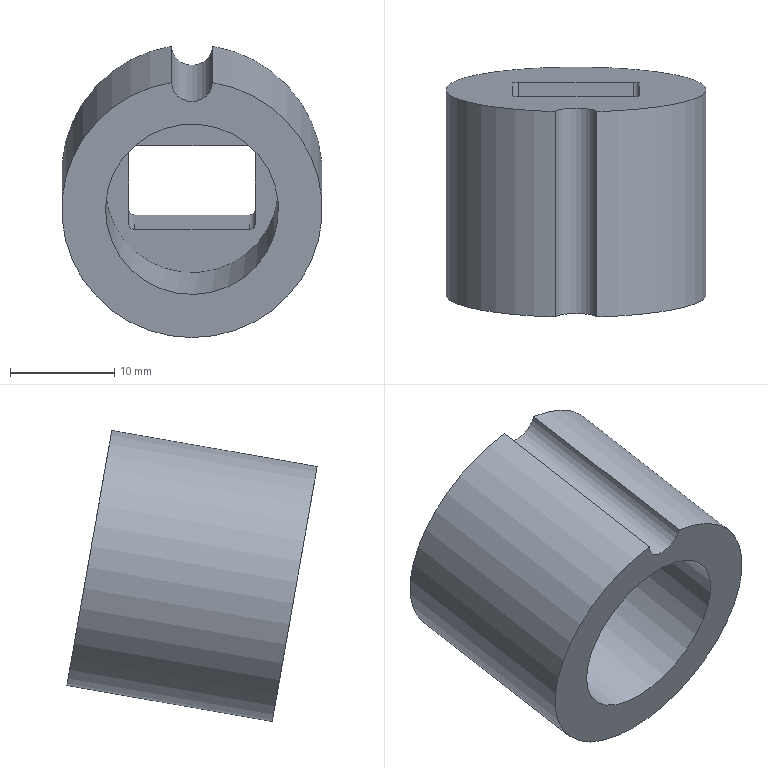Part | NX | features solid 2 | 1 solid | 14 faces | box 25 x 24.01 x 27.936 mm | volume 6304 mm3 | plane 7 | cylinder 7 | commonest cylinder face diameters 1.18 x4 4 x1 16.6 x1 25 x1
STEP:
#1=CARTESIAN_POINT('',(85.217,-526.176,-22.03));
#2=VERTEX_POINT('',#1);
#3=CARTESIAN_POINT('',(81.23,-526.176,-22.03));
#4=VERTEX_POINT('',#3);
#5=CARTESIAN_POINT('',(83.224,-526.203,-21.873));
#6=DIRECTION('',(0.,0.9848,0.1736));
#7=DIRECTION('',(-0.9972,0.01308,-0.07416));
#8=AXIS2_PLACEMENT_3D('',#5,#6,#7);
#9=CIRCLE('',#8,2.);
#10=EDGE_CURVE('',#2,#4,#9,.T.);
#11=ORIENTED_EDGE('',*,*,#10,.F.);
#12=CARTESIAN_POINT('',(83.224,-524.033,-34.183));
#13=DIRECTION('',(0.,0.9848,0.1736));
#14=DIRECTION('',(-0.9972,0.01308,-0.07416));
#15=AXIS2_PLACEMENT_3D('',#12,#13,#14);
#16=CIRCLE('',#15,12.5);
#17=EDGE_CURVE('',#2,#4,#16,.T.);
#18=ORIENTED_EDGE('',*,*,#17,.T.);
#19=EDGE_LOOP('',(#11,#18));
#20=FACE_BOUND('',#19,.T.);
#21=CARTESIAN_POINT('',(77.724,-524.743,-30.155));
#22=VERTEX_POINT('',#21);
#23=CARTESIAN_POINT('',(77.134,-524.641,-30.736));
#24=VERTEX_POINT('',#23);
#25=CARTESIAN_POINT('',(77.724,-524.641,-30.736));
#26=DIRECTION('',(0.,-0.9848,-0.1736));
#27=DIRECTION('',(0.,-0.1736,0.9848));
#28=AXIS2_PLACEMENT_3D('',#25,#26,#27);
#29=CIRCLE('',#28,0.59);
#30=EDGE_CURVE('',#22,#24,#29,.T.);
#31=ORIENTED_EDGE('',*,*,#30,.T.);
#32=CARTESIAN_POINT('',(77.134,-523.425,-37.63));
#33=VERTEX_POINT('',#32);
#34=CARTESIAN_POINT('',(77.134,-524.033,-34.183));
#35=DIRECTION('',(0.,-0.1736,0.9848));
#36=VECTOR('',#35,1000.);
#37=LINE('',#34,#36);
#38=EDGE_CURVE('',#33,#24,#37,.T.);
#39=ORIENTED_EDGE('',*,*,#38,.F.);
#40=CARTESIAN_POINT('',(77.724,-523.323,-38.211));
#41=VERTEX_POINT('',#40);
#42=CARTESIAN_POINT('',(77.724,-523.425,-37.63));
#43=DIRECTION('',(0.,-0.9848,-0.1736));
#44=DIRECTION('',(0.,-0.1736,0.9848));
#45=AXIS2_PLACEMENT_3D('',#42,#43,#44);
#46=CIRCLE('',#45,0.59);
#47=EDGE_CURVE('',#33,#41,#46,.T.);
#48=ORIENTED_EDGE('',*,*,#47,.T.);
#49=CARTESIAN_POINT('',(88.724,-523.323,-38.211));
#50=VERTEX_POINT('',#49);
#51=CARTESIAN_POINT('',(83.224,-523.323,-38.211));
#52=DIRECTION('',(-1.,0.,0.));
#53=VECTOR('',#52,1000.);
#54=LINE('',#51,#53);
#55=EDGE_CURVE('',#50,#41,#54,.T.);
#56=ORIENTED_EDGE('',*,*,#55,.F.);
#57=CARTESIAN_POINT('',(89.314,-523.425,-37.63));
#58=VERTEX_POINT('',#57);
#59=CARTESIAN_POINT('',(88.724,-523.425,-37.63));
#60=DIRECTION('',(0.,-0.9848,-0.1736));
#61=DIRECTION('',(0.,-0.1736,0.9848));
#62=AXIS2_PLACEMENT_3D('',#59,#60,#61);
#63=CIRCLE('',#62,0.59);
#64=EDGE_CURVE('',#50,#58,#63,.T.);
#65=ORIENTED_EDGE('',*,*,#64,.T.);
#66=CARTESIAN_POINT('',(89.314,-524.641,-30.736));
#67=VERTEX_POINT('',#66);
#68=CARTESIAN_POINT('',(89.314,-524.033,-34.183));
#69=DIRECTION('',(0.,0.1736,-0.9848));
#70=VECTOR('',#69,1000.);
#71=LINE('',#68,#70);
#72=EDGE_CURVE('',#67,#58,#71,.T.);
#73=ORIENTED_EDGE('',*,*,#72,.F.);
#74=CARTESIAN_POINT('',(88.724,-524.743,-30.155));
#75=VERTEX_POINT('',#74);
#76=CARTESIAN_POINT('',(88.724,-524.641,-30.736));
#77=DIRECTION('',(0.,-0.9848,-0.1736));
#78=DIRECTION('',(0.,-0.1736,0.9848));
#79=AXIS2_PLACEMENT_3D('',#76,#77,#78);
#80=CIRCLE('',#79,0.59);
#81=EDGE_CURVE('',#67,#75,#80,.T.);
#82=ORIENTED_EDGE('',*,*,#81,.T.);
#83=CARTESIAN_POINT('',(83.224,-524.743,-30.155));
#84=DIRECTION('',(1.,0.,0.));
#85=VECTOR('',#84,1000.);
#86=LINE('',#83,#85);
#87=EDGE_CURVE('',#22,#75,#86,.T.);
#88=ORIENTED_EDGE('',*,*,#87,.F.);
#89=EDGE_LOOP('',(#31,#39,#48,#56,#65,#73,#82,#88));
#90=FACE_BOUND('',#89,.T.);
#91=CARTESIAN_POINT('',(83.224,-524.033,-34.183));
#92=DIRECTION('',(0.,0.9848,0.1736));
#93=DIRECTION('',(0.9972,-0.01308,0.07416));
#94=AXIS2_PLACEMENT_3D('',#91,#92,#93);
#95=PLANE('',#94);
#96=ADVANCED_FACE('',(#20,#90),#95,.T.);
#97=CARTESIAN_POINT('',(81.23,-545.872,-25.503));
#98=VERTEX_POINT('',#97);
#99=CARTESIAN_POINT('',(85.217,-545.872,-25.503));
#100=VERTEX_POINT('',#99);
#101=CARTESIAN_POINT('',(83.224,-545.899,-25.346));
#102=DIRECTION('',(0.,-0.9848,-0.1736));
#103=DIRECTION('',(0.9972,-0.01308,0.07416));
#104=AXIS2_PLACEMENT_3D('',#101,#102,#103);
#105=CIRCLE('',#104,2.);
#106=EDGE_CURVE('',#98,#100,#105,.T.);
#107=ORIENTED_EDGE('',*,*,#106,.F.);
#108=CARTESIAN_POINT('',(83.224,-543.729,-37.656));
#109=DIRECTION('',(0.,-0.9848,-0.1736));
#110=DIRECTION('',(0.9972,-0.01308,0.07416));
#111=AXIS2_PLACEMENT_3D('',#108,#109,#110);
#112=CIRCLE('',#111,12.5);
#113=EDGE_CURVE('',#98,#100,#112,.T.);
#114=ORIENTED_EDGE('',*,*,#113,.T.);
#115=EDGE_LOOP('',(#107,#114));
#116=FACE_BOUND('',#115,.T.);
#117=CARTESIAN_POINT('',(91.5,-543.837,-37.04));
#118=VERTEX_POINT('',#117);
#119=CARTESIAN_POINT('',(83.224,-543.729,-37.656));
#120=DIRECTION('',(0.,-0.9848,-0.1736));
#121=DIRECTION('',(0.9972,-0.01308,0.07416));
#122=AXIS2_PLACEMENT_3D('',#119,#120,#121);
#123=CIRCLE('',#122,8.3);
#124=EDGE_CURVE('',#118,#118,#123,.T.);
#125=ORIENTED_EDGE('',*,*,#124,.F.);
#126=EDGE_LOOP('',(#125));
#127=FACE_BOUND('',#126,.T.);
#128=CARTESIAN_POINT('',(83.224,-543.729,-37.656));
#129=DIRECTION('',(0.,-0.9848,-0.1736));
#130=DIRECTION('',(-0.9972,0.01308,-0.07416));
#131=AXIS2_PLACEMENT_3D('',#128,#129,#130);
#132=PLANE('',#131);
#133=ADVANCED_FACE('',(#116,#127),#132,.T.);
#134=CARTESIAN_POINT('',(81.23,-536.024,-23.767));
#135=DIRECTION('',(0.,0.9848,0.1736));
#136=VECTOR('',#135,1000.);
#137=LINE('',#134,#136);
#138=EDGE_CURVE('',#98,#4,#137,.T.);
#139=ORIENTED_EDGE('',*,*,#138,.T.);
#140=ORIENTED_EDGE('',*,*,#17,.F.);
#141=CARTESIAN_POINT('',(85.217,-536.024,-23.767));
#142=DIRECTION('',(0.,0.9848,0.1736));
#143=VECTOR('',#142,1000.);
#144=LINE('',#141,#143);
#145=EDGE_CURVE('',#2,#100,#144,.F.);
#146=ORIENTED_EDGE('',*,*,#145,.T.);
#147=ORIENTED_EDGE('',*,*,#113,.F.);
#148=EDGE_LOOP('',(#139,#140,#146,#147));
#149=FACE_BOUND('',#148,.T.);
#150=CARTESIAN_POINT('',(83.224,-543.729,-37.656));
#151=DIRECTION('',(0.,0.9848,0.1736));
#152=DIRECTION('',(0.9972,-0.01308,0.07416));
#153=AXIS2_PLACEMENT_3D('',#150,#151,#152);
#154=CYLINDRICAL_SURFACE('',#153,12.5);
#155=ADVANCED_FACE('',(#149),#154,.T.);
#156=CARTESIAN_POINT('',(88.724,-532.621,-31.544));
#157=VERTEX_POINT('',#156);
#158=CARTESIAN_POINT('',(77.724,-532.621,-31.544));
#159=VERTEX_POINT('',#158);
#160=CARTESIAN_POINT('',(83.224,-532.621,-31.544));
#161=DIRECTION('',(-1.,0.,0.));
#162=VECTOR('',#161,1000.);
#163=LINE('',#160,#162);
#164=EDGE_CURVE('',#157,#159,#163,.T.);
#165=ORIENTED_EDGE('',*,*,#164,.F.);
#166=CARTESIAN_POINT('',(89.314,-532.519,-32.125));
#167=VERTEX_POINT('',#166);
#168=CARTESIAN_POINT('',(88.724,-532.519,-32.125));
#169=DIRECTION('',(0.,0.9848,0.1736));
#170=DIRECTION('',(0.,0.1736,-0.9848));
#171=AXIS2_PLACEMENT_3D('',#168,#169,#170);
#172=CIRCLE('',#171,0.59);
#173=EDGE_CURVE('',#157,#167,#172,.T.);
#174=ORIENTED_EDGE('',*,*,#173,.T.);
#175=CARTESIAN_POINT('',(89.314,-531.303,-39.019));
#176=VERTEX_POINT('',#175);
#177=CARTESIAN_POINT('',(89.314,-531.911,-35.572));
#178=DIRECTION('',(0.,-0.1736,0.9848));
#179=VECTOR('',#178,1000.);
#180=LINE('',#177,#179);
#181=EDGE_CURVE('',#176,#167,#180,.T.);
#182=ORIENTED_EDGE('',*,*,#181,.F.);
#183=CARTESIAN_POINT('',(88.724,-531.201,-39.6));
#184=VERTEX_POINT('',#183);
#185=CARTESIAN_POINT('',(88.724,-531.303,-39.019));
#186=DIRECTION('',(0.,0.9848,0.1736));
#187=DIRECTION('',(0.,0.1736,-0.9848));
#188=AXIS2_PLACEMENT_3D('',#185,#186,#187);
#189=CIRCLE('',#188,0.59);
#190=EDGE_CURVE('',#176,#184,#189,.T.);
#191=ORIENTED_EDGE('',*,*,#190,.T.);
#192=CARTESIAN_POINT('',(77.724,-531.201,-39.6));
#193=VERTEX_POINT('',#192);
#194=CARTESIAN_POINT('',(83.224,-531.201,-39.6));
#195=DIRECTION('',(1.,0.,0.));
#196=VECTOR('',#195,1000.);
#197=LINE('',#194,#196);
#198=EDGE_CURVE('',#193,#184,#197,.T.);
#199=ORIENTED_EDGE('',*,*,#198,.F.);
#200=CARTESIAN_POINT('',(77.134,-531.303,-39.019));
#201=VERTEX_POINT('',#200);
#202=CARTESIAN_POINT('',(77.724,-531.303,-39.019));
#203=DIRECTION('',(0.,0.9848,0.1736));
#204=DIRECTION('',(0.,0.1736,-0.9848));
#205=AXIS2_PLACEMENT_3D('',#202,#203,#204);
#206=CIRCLE('',#205,0.59);
#207=EDGE_CURVE('',#193,#201,#206,.T.);
#208=ORIENTED_EDGE('',*,*,#207,.T.);
#209=CARTESIAN_POINT('',(77.134,-532.519,-32.125));
#210=VERTEX_POINT('',#209);
#211=CARTESIAN_POINT('',(77.134,-531.911,-35.572));
#212=DIRECTION('',(0.,0.1736,-0.9848));
#213=VECTOR('',#212,1000.);
#214=LINE('',#211,#213);
#215=EDGE_CURVE('',#210,#201,#214,.T.);
#216=ORIENTED_EDGE('',*,*,#215,.F.);
#217=CARTESIAN_POINT('',(77.724,-532.519,-32.125));
#218=DIRECTION('',(0.,0.9848,0.1736));
#219=DIRECTION('',(0.,0.1736,-0.9848));
#220=AXIS2_PLACEMENT_3D('',#217,#218,#219);
#221=CIRCLE('',#220,0.59);
#222=EDGE_CURVE('',#210,#159,#221,.T.);
#223=ORIENTED_EDGE('',*,*,#222,.T.);
#224=EDGE_LOOP('',(#165,#174,#182,#191,#199,#208,#216,#223));
#225=FACE_BOUND('',#224,.T.);
#226=CARTESIAN_POINT('',(74.947,-531.803,-36.188));
#227=VERTEX_POINT('',#226);
#228=CARTESIAN_POINT('',(83.224,-531.911,-35.572));
#229=DIRECTION('',(0.,0.9848,0.1736));
#230=DIRECTION('',(-0.9972,0.01308,-0.07416));
#231=AXIS2_PLACEMENT_3D('',#228,#229,#230);
#232=CIRCLE('',#231,8.3);
#233=EDGE_CURVE('',#227,#227,#232,.T.);
#234=ORIENTED_EDGE('',*,*,#233,.F.);
#235=EDGE_LOOP('',(#234));
#236=FACE_BOUND('',#235,.T.);
#237=CARTESIAN_POINT('',(83.224,-531.911,-35.572));
#238=DIRECTION('',(0.,0.9848,0.1736));
#239=DIRECTION('',(0.9972,-0.01308,0.07416));
#240=AXIS2_PLACEMENT_3D('',#237,#238,#239);
#241=PLANE('',#240);
#242=ADVANCED_FACE('',(#225,#236),#241,.F.);
#243=ORIENTED_EDGE('',*,*,#233,.T.);
#244=EDGE_LOOP('',(#243));
#245=FACE_BOUND('',#244,.T.);
#246=ORIENTED_EDGE('',*,*,#124,.T.);
#247=EDGE_LOOP('',(#246));
#248=FACE_BOUND('',#247,.T.);
#249=CARTESIAN_POINT('',(83.224,-543.729,-37.656));
#250=DIRECTION('',(0.,0.9848,0.1736));
#251=DIRECTION('',(0.9972,-0.01308,0.07416));
#252=AXIS2_PLACEMENT_3D('',#249,#250,#251);
#253=CYLINDRICAL_SURFACE('',#252,8.3);
#254=ADVANCED_FACE('',(#245,#248),#253,.F.);
#255=ORIENTED_EDGE('',*,*,#181,.T.);
#256=CARTESIAN_POINT('',(89.314,-532.519,-32.125));
#257=DIRECTION('',(0.,0.9848,0.1736));
#258=VECTOR('',#257,1000.);
#259=LINE('',#256,#258);
#260=EDGE_CURVE('',#167,#67,#259,.T.);
#261=ORIENTED_EDGE('',*,*,#260,.T.);
#262=ORIENTED_EDGE('',*,*,#72,.T.);
#263=CARTESIAN_POINT('',(89.314,-531.303,-39.019));
#264=DIRECTION('',(0.,0.9848,0.1736));
#265=VECTOR('',#264,1000.);
#266=LINE('',#263,#265);
#267=EDGE_CURVE('',#58,#176,#266,.F.);
#268=ORIENTED_EDGE('',*,*,#267,.T.);
#269=EDGE_LOOP('',(#255,#261,#262,#268));
#270=FACE_BOUND('',#269,.T.);
#271=CARTESIAN_POINT('',(89.314,-531.911,-35.572));
#272=DIRECTION('',(1.,0.,0.));
#273=DIRECTION('',(0.,-0.9848,-0.1736));
#274=AXIS2_PLACEMENT_3D('',#271,#272,#273);
#275=PLANE('',#274);
#276=ADVANCED_FACE('',(#270),#275,.F.);
#277=ORIENTED_EDGE('',*,*,#55,.T.);
#278=CARTESIAN_POINT('',(77.724,-531.201,-39.6));
#279=DIRECTION('',(0.,0.9848,0.1736));
#280=VECTOR('',#279,1000.);
#281=LINE('',#278,#280);
#282=EDGE_CURVE('',#41,#193,#281,.F.);
#283=ORIENTED_EDGE('',*,*,#282,.T.);
#284=ORIENTED_EDGE('',*,*,#198,.T.);
#285=CARTESIAN_POINT('',(88.724,-531.201,-39.6));
#286=DIRECTION('',(0.,0.9848,0.1736));
#287=VECTOR('',#286,1000.);
#288=LINE('',#285,#287);
#289=EDGE_CURVE('',#184,#50,#288,.T.);
#290=ORIENTED_EDGE('',*,*,#289,.T.);
#291=EDGE_LOOP('',(#277,#283,#284,#290));
#292=FACE_BOUND('',#291,.T.);
#293=CARTESIAN_POINT('',(83.224,-531.201,-39.6));
#294=DIRECTION('',(0.,0.1736,-0.9848));
#295=DIRECTION('',(0.,0.9848,0.1736));
#296=AXIS2_PLACEMENT_3D('',#293,#294,#295);
#297=PLANE('',#296);
#298=ADVANCED_FACE('',(#292),#297,.F.);
#299=ORIENTED_EDGE('',*,*,#38,.T.);
#300=CARTESIAN_POINT('',(77.134,-532.519,-32.125));
#301=DIRECTION('',(0.,0.9848,0.1736));
#302=VECTOR('',#301,1000.);
#303=LINE('',#300,#302);
#304=EDGE_CURVE('',#24,#210,#303,.F.);
#305=ORIENTED_EDGE('',*,*,#304,.T.);
#306=ORIENTED_EDGE('',*,*,#215,.T.);
#307=CARTESIAN_POINT('',(77.134,-531.303,-39.019));
#308=DIRECTION('',(0.,0.9848,0.1736));
#309=VECTOR('',#308,1000.);
#310=LINE('',#307,#309);
#311=EDGE_CURVE('',#201,#33,#310,.T.);
#312=ORIENTED_EDGE('',*,*,#311,.T.);
#313=EDGE_LOOP('',(#299,#305,#306,#312));
#314=FACE_BOUND('',#313,.T.);
#315=CARTESIAN_POINT('',(77.134,-531.911,-35.572));
#316=DIRECTION('',(-1.,0.,0.));
#317=DIRECTION('',(0.,0.9848,0.1736));
#318=AXIS2_PLACEMENT_3D('',#315,#316,#317);
#319=PLANE('',#318);
#320=ADVANCED_FACE('',(#314),#319,.F.);
#321=ORIENTED_EDGE('',*,*,#87,.T.);
#322=CARTESIAN_POINT('',(88.724,-532.621,-31.544));
#323=DIRECTION('',(0.,0.9848,0.1736));
#324=VECTOR('',#323,1000.);
#325=LINE('',#322,#324);
#326=EDGE_CURVE('',#75,#157,#325,.F.);
#327=ORIENTED_EDGE('',*,*,#326,.T.);
#328=ORIENTED_EDGE('',*,*,#164,.T.);
#329=CARTESIAN_POINT('',(77.724,-532.621,-31.544));
#330=DIRECTION('',(0.,0.9848,0.1736));
#331=VECTOR('',#330,1000.);
#332=LINE('',#329,#331);
#333=EDGE_CURVE('',#159,#22,#332,.T.);
#334=ORIENTED_EDGE('',*,*,#333,.T.);
#335=EDGE_LOOP('',(#321,#327,#328,#334));
#336=FACE_BOUND('',#335,.T.);
#337=CARTESIAN_POINT('',(83.224,-532.621,-31.544));
#338=DIRECTION('',(0.,-0.1736,0.9848));
#339=DIRECTION('',(0.,-0.9848,-0.1736));
#340=AXIS2_PLACEMENT_3D('',#337,#338,#339);
#341=PLANE('',#340);
#342=ADVANCED_FACE('',(#336),#341,.F.);
#343=ORIENTED_EDGE('',*,*,#173,.F.);
#344=ORIENTED_EDGE('',*,*,#326,.F.);
#345=ORIENTED_EDGE('',*,*,#81,.F.);
#346=ORIENTED_EDGE('',*,*,#260,.F.);
#347=EDGE_LOOP('',(#343,#344,#345,#346));
#348=FACE_BOUND('',#347,.T.);
#349=CARTESIAN_POINT('',(88.724,-532.519,-32.125));
#350=DIRECTION('',(0.,0.9848,0.1736));
#351=DIRECTION('',(0.,-0.1736,0.9848));
#352=AXIS2_PLACEMENT_3D('',#349,#350,#351);
#353=CYLINDRICAL_SURFACE('',#352,0.59);
#354=ADVANCED_FACE('',(#348),#353,.F.);
#355=ORIENTED_EDGE('',*,*,#222,.F.);
#356=ORIENTED_EDGE('',*,*,#304,.F.);
#357=ORIENTED_EDGE('',*,*,#30,.F.);
#358=ORIENTED_EDGE('',*,*,#333,.F.);
#359=EDGE_LOOP('',(#355,#356,#357,#358));
#360=FACE_BOUND('',#359,.T.);
#361=CARTESIAN_POINT('',(77.724,-532.519,-32.125));
#362=DIRECTION('',(0.,0.9848,0.1736));
#363=DIRECTION('',(0.,-0.1736,0.9848));
#364=AXIS2_PLACEMENT_3D('',#361,#362,#363);
#365=CYLINDRICAL_SURFACE('',#364,0.59);
#366=ADVANCED_FACE('',(#360),#365,.F.);
#367=ORIENTED_EDGE('',*,*,#207,.F.);
#368=ORIENTED_EDGE('',*,*,#282,.F.);
#369=ORIENTED_EDGE('',*,*,#47,.F.);
#370=ORIENTED_EDGE('',*,*,#311,.F.);
#371=EDGE_LOOP('',(#367,#368,#369,#370));
#372=FACE_BOUND('',#371,.T.);
#373=CARTESIAN_POINT('',(77.724,-531.303,-39.019));
#374=DIRECTION('',(0.,0.9848,0.1736));
#375=DIRECTION('',(0.,-0.1736,0.9848));
#376=AXIS2_PLACEMENT_3D('',#373,#374,#375);
#377=CYLINDRICAL_SURFACE('',#376,0.59);
#378=ADVANCED_FACE('',(#372),#377,.F.);
#379=ORIENTED_EDGE('',*,*,#190,.F.);
#380=ORIENTED_EDGE('',*,*,#267,.F.);
#381=ORIENTED_EDGE('',*,*,#64,.F.);
#382=ORIENTED_EDGE('',*,*,#289,.F.);
#383=EDGE_LOOP('',(#379,#380,#381,#382));
#384=FACE_BOUND('',#383,.T.);
#385=CARTESIAN_POINT('',(88.724,-531.303,-39.019));
#386=DIRECTION('',(0.,0.9848,0.1736));
#387=DIRECTION('',(0.,-0.1736,0.9848));
#388=AXIS2_PLACEMENT_3D('',#385,#386,#387);
#389=CYLINDRICAL_SURFACE('',#388,0.59);
#390=ADVANCED_FACE('',(#384),#389,.F.);
#391=ORIENTED_EDGE('',*,*,#138,.F.);
#392=ORIENTED_EDGE('',*,*,#106,.T.);
#393=ORIENTED_EDGE('',*,*,#145,.F.);
#394=ORIENTED_EDGE('',*,*,#10,.T.);
#395=EDGE_LOOP('',(#391,#392,#393,#394));
#396=FACE_BOUND('',#395,.T.);
#397=CARTESIAN_POINT('',(83.224,-545.899,-25.346));
#398=DIRECTION('',(0.,0.9848,0.1736));
#399=DIRECTION('',(0.9972,-0.01308,0.07416));
#400=AXIS2_PLACEMENT_3D('',#397,#398,#399);
#401=CYLINDRICAL_SURFACE('',#400,2.);
#402=ADVANCED_FACE('',(#396),#401,.F.);
#403=CLOSED_SHELL('',(#96,#133,#155,#242,#254,#276,#298,#320,#342,#354,#366,#378,#390,#402));
#404=MANIFOLD_SOLID_BREP('',#403);
#405=(LENGTH_UNIT()NAMED_UNIT(*)SI_UNIT(.MILLI.,.METRE.));
#406=UNCERTAINTY_MEASURE_WITH_UNIT(LENGTH_MEASURE(0.00001),#405,'','');
#407=(NAMED_UNIT(*)PLANE_ANGLE_UNIT()SI_UNIT($,.RADIAN.));
#408=(NAMED_UNIT(*)SI_UNIT($,.STERADIAN.)SOLID_ANGLE_UNIT());
#409=(GEOMETRIC_REPRESENTATION_CONTEXT(3)GLOBAL_UNCERTAINTY_ASSIGNED_CONTEXT((#406))GLOBAL_UNIT_ASSIGNED_CONTEXT((#405,#407,#408))REPRESENTATION_CONTEXT('',''));
#410=ADVANCED_BREP_SHAPE_REPRESENTATION('',(#404),#409);